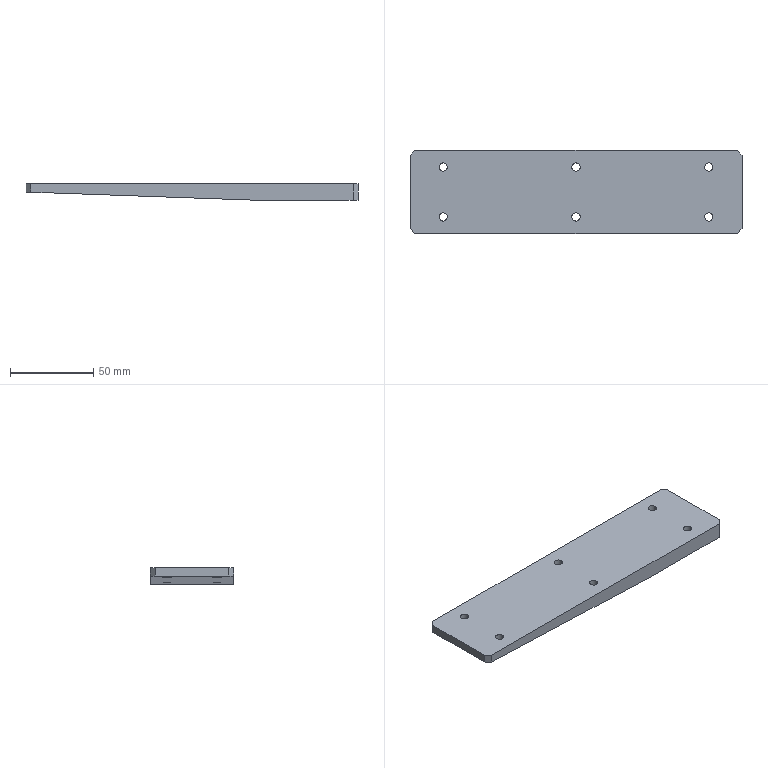Part | SolidWorks | features BaseBody 1 | 1 solid | 23 faces | box 200 x 50 x 10 mm | volume 81411 mm3 | cylinder 12 | plane 11 | commonest cylinder face diameters 5 x12
STEP:
#1=CARTESIAN_POINT('',(-82.5,15.,-0.625));
#2=VERTEX_POINT('',#1);
#3=CARTESIAN_POINT('',(-77.5,15.,-0.8036));
#4=VERTEX_POINT('',#3);
#5=CARTESIAN_POINT('',(-82.5,15.,-0.625));
#6=CARTESIAN_POINT('',(-82.5,10.,-0.625));
#7=CARTESIAN_POINT('',(-77.5,10.,-0.8036));
#8=CARTESIAN_POINT('',(-77.5,15.,-0.8036));
#9=(BOUNDED_CURVE()B_SPLINE_CURVE(3,(#5,#6,#7,#8),.UNSPECIFIED.,.F.,.F.)B_SPLINE_CURVE_WITH_KNOTS((4,4),(0.,3.142),.UNSPECIFIED.)CURVE()GEOMETRIC_REPRESENTATION_ITEM()RATIONAL_B_SPLINE_CURVE((1.,0.3333,0.3333,1.))REPRESENTATION_ITEM(''));
#10=EDGE_CURVE('',#2,#4,#9,.T.);
#11=ORIENTED_EDGE('',*,*,#10,.F.);
#12=CARTESIAN_POINT('',(-82.5,15.,5.));
#13=VERTEX_POINT('',#12);
#14=CARTESIAN_POINT('',(-82.5,15.,5.));
#15=DIRECTION('',(0.,0.,1.));
#16=VECTOR('',#15,1000.);
#17=LINE('',#14,#16);
#18=EDGE_CURVE('',#2,#13,#17,.T.);
#19=ORIENTED_EDGE('',*,*,#18,.T.);
#20=CARTESIAN_POINT('',(-77.5,15.,5.));
#21=VERTEX_POINT('',#20);
#22=CARTESIAN_POINT('',(-80.,15.,5.));
#23=DIRECTION('',(0.,0.,1.));
#24=DIRECTION('',(1.,0.,0.));
#25=AXIS2_PLACEMENT_3D('',#22,#23,#24);
#26=CIRCLE('',#25,2.5);
#27=EDGE_CURVE('',#13,#21,#26,.T.);
#28=ORIENTED_EDGE('',*,*,#27,.T.);
#29=CARTESIAN_POINT('',(-77.5,15.,5.));
#30=DIRECTION('',(0.,0.,1.));
#31=VECTOR('',#30,1000.);
#32=LINE('',#29,#31);
#33=EDGE_CURVE('',#4,#21,#32,.T.);
#34=ORIENTED_EDGE('',*,*,#33,.F.);
#35=EDGE_LOOP('',(#11,#19,#28,#34));
#36=FACE_OUTER_BOUND('',#35,.T.);
#37=CARTESIAN_POINT('',(-80.,15.,5.));
#38=DIRECTION('',(0.,0.,1.));
#39=DIRECTION('',(1.,0.,0.));
#40=AXIS2_PLACEMENT_3D('',#37,#38,#39);
#41=CYLINDRICAL_SURFACE('',#40,2.5);
#42=ADVANCED_FACE('',(#36),#41,.F.);
#43=CARTESIAN_POINT('',(-82.5,-15.,-0.625));
#44=VERTEX_POINT('',#43);
#45=CARTESIAN_POINT('',(-77.5,-15.,-0.8036));
#46=VERTEX_POINT('',#45);
#47=CARTESIAN_POINT('',(-82.5,-15.,-0.625));
#48=CARTESIAN_POINT('',(-82.5,-20.,-0.625));
#49=CARTESIAN_POINT('',(-77.5,-20.,-0.8036));
#50=CARTESIAN_POINT('',(-77.5,-15.,-0.8036));
#51=(BOUNDED_CURVE()B_SPLINE_CURVE(3,(#47,#48,#49,#50),.UNSPECIFIED.,.F.,.F.)B_SPLINE_CURVE_WITH_KNOTS((4,4),(0.,3.142),.UNSPECIFIED.)CURVE()GEOMETRIC_REPRESENTATION_ITEM()RATIONAL_B_SPLINE_CURVE((1.,0.3333,0.3333,1.))REPRESENTATION_ITEM(''));
#52=EDGE_CURVE('',#44,#46,#51,.T.);
#53=ORIENTED_EDGE('',*,*,#52,.F.);
#54=CARTESIAN_POINT('',(-82.5,-15.,5.));
#55=VERTEX_POINT('',#54);
#56=CARTESIAN_POINT('',(-82.5,-15.,5.));
#57=DIRECTION('',(0.,0.,1.));
#58=VECTOR('',#57,1000.);
#59=LINE('',#56,#58);
#60=EDGE_CURVE('',#44,#55,#59,.T.);
#61=ORIENTED_EDGE('',*,*,#60,.T.);
#62=CARTESIAN_POINT('',(-77.5,-15.,5.));
#63=VERTEX_POINT('',#62);
#64=CARTESIAN_POINT('',(-80.,-15.,5.));
#65=DIRECTION('',(0.,0.,1.));
#66=DIRECTION('',(1.,0.,0.));
#67=AXIS2_PLACEMENT_3D('',#64,#65,#66);
#68=CIRCLE('',#67,2.5);
#69=EDGE_CURVE('',#55,#63,#68,.T.);
#70=ORIENTED_EDGE('',*,*,#69,.T.);
#71=CARTESIAN_POINT('',(-77.5,-15.,5.));
#72=DIRECTION('',(0.,0.,1.));
#73=VECTOR('',#72,1000.);
#74=LINE('',#71,#73);
#75=EDGE_CURVE('',#46,#63,#74,.T.);
#76=ORIENTED_EDGE('',*,*,#75,.F.);
#77=EDGE_LOOP('',(#53,#61,#70,#76));
#78=FACE_OUTER_BOUND('',#77,.T.);
#79=CARTESIAN_POINT('',(-80.,-15.,5.));
#80=DIRECTION('',(0.,0.,1.));
#81=DIRECTION('',(1.,0.,0.));
#82=AXIS2_PLACEMENT_3D('',#79,#80,#81);
#83=CYLINDRICAL_SURFACE('',#82,2.5);
#84=ADVANCED_FACE('',(#78),#83,.F.);
#85=CARTESIAN_POINT('',(-2.5,15.,-3.482));
#86=VERTEX_POINT('',#85);
#87=CARTESIAN_POINT('',(2.5,15.,-3.661));
#88=VERTEX_POINT('',#87);
#89=CARTESIAN_POINT('',(-2.5,15.,-3.482));
#90=CARTESIAN_POINT('',(-2.5,10.,-3.482));
#91=CARTESIAN_POINT('',(2.5,10.,-3.661));
#92=CARTESIAN_POINT('',(2.5,15.,-3.661));
#93=(BOUNDED_CURVE()B_SPLINE_CURVE(3,(#89,#90,#91,#92),.UNSPECIFIED.,.F.,.T.)B_SPLINE_CURVE_WITH_KNOTS((4,4),(0.,3.142),.UNSPECIFIED.)CURVE()GEOMETRIC_REPRESENTATION_ITEM()RATIONAL_B_SPLINE_CURVE((1.,0.3333,0.3333,1.))REPRESENTATION_ITEM(''));
#94=EDGE_CURVE('',#86,#88,#93,.T.);
#95=ORIENTED_EDGE('',*,*,#94,.F.);
#96=CARTESIAN_POINT('',(-2.5,15.,5.));
#97=VERTEX_POINT('',#96);
#98=CARTESIAN_POINT('',(-2.5,15.,5.));
#99=DIRECTION('',(0.,0.,1.));
#100=VECTOR('',#99,1000.);
#101=LINE('',#98,#100);
#102=EDGE_CURVE('',#86,#97,#101,.T.);
#103=ORIENTED_EDGE('',*,*,#102,.T.);
#104=CARTESIAN_POINT('',(2.5,15.,5.));
#105=VERTEX_POINT('',#104);
#106=CARTESIAN_POINT('',(0.,15.,5.));
#107=DIRECTION('',(0.,0.,1.));
#108=DIRECTION('',(1.,0.,0.));
#109=AXIS2_PLACEMENT_3D('',#106,#107,#108);
#110=CIRCLE('',#109,2.5);
#111=EDGE_CURVE('',#97,#105,#110,.T.);
#112=ORIENTED_EDGE('',*,*,#111,.T.);
#113=CARTESIAN_POINT('',(2.5,15.,5.));
#114=DIRECTION('',(0.,0.,1.));
#115=VECTOR('',#114,1000.);
#116=LINE('',#113,#115);
#117=EDGE_CURVE('',#88,#105,#116,.T.);
#118=ORIENTED_EDGE('',*,*,#117,.F.);
#119=EDGE_LOOP('',(#95,#103,#112,#118));
#120=FACE_OUTER_BOUND('',#119,.T.);
#121=CARTESIAN_POINT('',(0.,15.,5.));
#122=DIRECTION('',(0.,0.,1.));
#123=DIRECTION('',(1.,0.,0.));
#124=AXIS2_PLACEMENT_3D('',#121,#122,#123);
#125=CYLINDRICAL_SURFACE('',#124,2.5);
#126=ADVANCED_FACE('',(#120),#125,.F.);
#127=CARTESIAN_POINT('',(-2.5,-15.,-3.482));
#128=VERTEX_POINT('',#127);
#129=CARTESIAN_POINT('',(2.5,-15.,-3.661));
#130=VERTEX_POINT('',#129);
#131=CARTESIAN_POINT('',(-2.5,-15.,-3.482));
#132=CARTESIAN_POINT('',(-2.5,-20.,-3.482));
#133=CARTESIAN_POINT('',(2.5,-20.,-3.661));
#134=CARTESIAN_POINT('',(2.5,-15.,-3.661));
#135=(BOUNDED_CURVE()B_SPLINE_CURVE(3,(#131,#132,#133,#134),.UNSPECIFIED.,.F.,.F.)B_SPLINE_CURVE_WITH_KNOTS((4,4),(0.,3.142),.UNSPECIFIED.)CURVE()GEOMETRIC_REPRESENTATION_ITEM()RATIONAL_B_SPLINE_CURVE((1.,0.3333,0.3333,1.))REPRESENTATION_ITEM(''));
#136=EDGE_CURVE('',#128,#130,#135,.T.);
#137=ORIENTED_EDGE('',*,*,#136,.F.);
#138=CARTESIAN_POINT('',(-2.5,-15.,5.));
#139=VERTEX_POINT('',#138);
#140=CARTESIAN_POINT('',(-2.5,-15.,5.));
#141=DIRECTION('',(0.,0.,1.));
#142=VECTOR('',#141,1000.);
#143=LINE('',#140,#142);
#144=EDGE_CURVE('',#128,#139,#143,.T.);
#145=ORIENTED_EDGE('',*,*,#144,.T.);
#146=CARTESIAN_POINT('',(2.5,-15.,5.));
#147=VERTEX_POINT('',#146);
#148=CARTESIAN_POINT('',(0.,-15.,5.));
#149=DIRECTION('',(0.,0.,1.));
#150=DIRECTION('',(1.,0.,0.));
#151=AXIS2_PLACEMENT_3D('',#148,#149,#150);
#152=CIRCLE('',#151,2.5);
#153=EDGE_CURVE('',#139,#147,#152,.T.);
#154=ORIENTED_EDGE('',*,*,#153,.T.);
#155=CARTESIAN_POINT('',(2.5,-15.,5.));
#156=DIRECTION('',(0.,0.,1.));
#157=VECTOR('',#156,1000.);
#158=LINE('',#155,#157);
#159=EDGE_CURVE('',#130,#147,#158,.T.);
#160=ORIENTED_EDGE('',*,*,#159,.F.);
#161=EDGE_LOOP('',(#137,#145,#154,#160));
#162=FACE_OUTER_BOUND('',#161,.T.);
#163=CARTESIAN_POINT('',(0.,-15.,5.));
#164=DIRECTION('',(0.,0.,1.));
#165=DIRECTION('',(1.,0.,0.));
#166=AXIS2_PLACEMENT_3D('',#163,#164,#165);
#167=CYLINDRICAL_SURFACE('',#166,2.5);
#168=ADVANCED_FACE('',(#162),#167,.F.);
#169=CARTESIAN_POINT('',(82.5,15.,-5.));
#170=VERTEX_POINT('',#169);
#171=CARTESIAN_POINT('',(77.5,15.,-5.));
#172=VERTEX_POINT('',#171);
#173=CARTESIAN_POINT('',(80.,15.,-5.));
#174=DIRECTION('',(0.,0.,-1.));
#175=DIRECTION('',(-1.,0.,0.));
#176=AXIS2_PLACEMENT_3D('',#173,#174,#175);
#177=CIRCLE('',#176,2.5);
#178=EDGE_CURVE('',#170,#172,#177,.T.);
#179=ORIENTED_EDGE('',*,*,#178,.T.);
#180=CARTESIAN_POINT('',(77.5,15.,5.));
#181=VERTEX_POINT('',#180);
#182=CARTESIAN_POINT('',(77.5,15.,5.));
#183=DIRECTION('',(0.,0.,1.));
#184=VECTOR('',#183,1000.);
#185=LINE('',#182,#184);
#186=EDGE_CURVE('',#172,#181,#185,.T.);
#187=ORIENTED_EDGE('',*,*,#186,.T.);
#188=CARTESIAN_POINT('',(82.5,15.,5.));
#189=VERTEX_POINT('',#188);
#190=CARTESIAN_POINT('',(80.,15.,5.));
#191=DIRECTION('',(0.,0.,1.));
#192=DIRECTION('',(1.,0.,0.));
#193=AXIS2_PLACEMENT_3D('',#190,#191,#192);
#194=CIRCLE('',#193,2.5);
#195=EDGE_CURVE('',#181,#189,#194,.T.);
#196=ORIENTED_EDGE('',*,*,#195,.T.);
#197=CARTESIAN_POINT('',(82.5,15.,5.));
#198=DIRECTION('',(0.,0.,1.));
#199=VECTOR('',#198,1000.);
#200=LINE('',#197,#199);
#201=EDGE_CURVE('',#170,#189,#200,.T.);
#202=ORIENTED_EDGE('',*,*,#201,.F.);
#203=EDGE_LOOP('',(#179,#187,#196,#202));
#204=FACE_OUTER_BOUND('',#203,.T.);
#205=CARTESIAN_POINT('',(80.,15.,5.));
#206=DIRECTION('',(0.,0.,1.));
#207=DIRECTION('',(1.,0.,0.));
#208=AXIS2_PLACEMENT_3D('',#205,#206,#207);
#209=CYLINDRICAL_SURFACE('',#208,2.5);
#210=ADVANCED_FACE('',(#204),#209,.F.);
#211=CARTESIAN_POINT('',(82.5,-15.,-5.));
#212=VERTEX_POINT('',#211);
#213=CARTESIAN_POINT('',(77.5,-15.,-5.));
#214=VERTEX_POINT('',#213);
#215=CARTESIAN_POINT('',(80.,-15.,-5.));
#216=DIRECTION('',(0.,0.,-1.));
#217=DIRECTION('',(-1.,0.,0.));
#218=AXIS2_PLACEMENT_3D('',#215,#216,#217);
#219=CIRCLE('',#218,2.5);
#220=EDGE_CURVE('',#212,#214,#219,.T.);
#221=ORIENTED_EDGE('',*,*,#220,.T.);
#222=CARTESIAN_POINT('',(77.5,-15.,5.));
#223=VERTEX_POINT('',#222);
#224=CARTESIAN_POINT('',(77.5,-15.,5.));
#225=DIRECTION('',(0.,0.,1.));
#226=VECTOR('',#225,1000.);
#227=LINE('',#224,#226);
#228=EDGE_CURVE('',#214,#223,#227,.T.);
#229=ORIENTED_EDGE('',*,*,#228,.T.);
#230=CARTESIAN_POINT('',(82.5,-15.,5.));
#231=VERTEX_POINT('',#230);
#232=CARTESIAN_POINT('',(80.,-15.,5.));
#233=DIRECTION('',(0.,0.,1.));
#234=DIRECTION('',(1.,0.,0.));
#235=AXIS2_PLACEMENT_3D('',#232,#233,#234);
#236=CIRCLE('',#235,2.5);
#237=EDGE_CURVE('',#223,#231,#236,.T.);
#238=ORIENTED_EDGE('',*,*,#237,.T.);
#239=CARTESIAN_POINT('',(82.5,-15.,5.));
#240=DIRECTION('',(0.,0.,1.));
#241=VECTOR('',#240,1000.);
#242=LINE('',#239,#241);
#243=EDGE_CURVE('',#212,#231,#242,.T.);
#244=ORIENTED_EDGE('',*,*,#243,.F.);
#245=EDGE_LOOP('',(#221,#229,#238,#244));
#246=FACE_OUTER_BOUND('',#245,.T.);
#247=CARTESIAN_POINT('',(80.,-15.,5.));
#248=DIRECTION('',(0.,0.,1.));
#249=DIRECTION('',(1.,0.,0.));
#250=AXIS2_PLACEMENT_3D('',#247,#248,#249);
#251=CYLINDRICAL_SURFACE('',#250,2.5);
#252=ADVANCED_FACE('',(#246),#251,.F.);
#253=CARTESIAN_POINT('',(-100.,-22.,0.));
#254=VERTEX_POINT('',#253);
#255=CARTESIAN_POINT('',(-100.,22.,0.));
#256=VERTEX_POINT('',#255);
#257=CARTESIAN_POINT('',(-100.,-25.,0.));
#258=DIRECTION('',(0.,1.,0.));
#259=VECTOR('',#258,1000.);
#260=LINE('',#257,#259);
#261=EDGE_CURVE('',#254,#256,#260,.T.);
#262=ORIENTED_EDGE('',*,*,#261,.F.);
#263=CARTESIAN_POINT('',(-100.,-22.,5.));
#264=VERTEX_POINT('',#263);
#265=CARTESIAN_POINT('',(-100.,-22.,5.));
#266=DIRECTION('',(0.,0.,1.));
#267=VECTOR('',#266,1000.);
#268=LINE('',#265,#267);
#269=EDGE_CURVE('',#254,#264,#268,.T.);
#270=ORIENTED_EDGE('',*,*,#269,.T.);
#271=CARTESIAN_POINT('',(-100.,22.,5.));
#272=VERTEX_POINT('',#271);
#273=CARTESIAN_POINT('',(-100.,25.,5.));
#274=DIRECTION('',(0.,-1.,0.));
#275=VECTOR('',#274,1000.);
#276=LINE('',#273,#275);
#277=EDGE_CURVE('',#272,#264,#276,.T.);
#278=ORIENTED_EDGE('',*,*,#277,.F.);
#279=CARTESIAN_POINT('',(-100.,22.,5.));
#280=DIRECTION('',(0.,0.,-1.));
#281=VECTOR('',#280,1000.);
#282=LINE('',#279,#281);
#283=EDGE_CURVE('',#272,#256,#282,.T.);
#284=ORIENTED_EDGE('',*,*,#283,.T.);
#285=EDGE_LOOP('',(#262,#270,#278,#284));
#286=FACE_OUTER_BOUND('',#285,.T.);
#287=CARTESIAN_POINT('',(-100.,25.,5.));
#288=DIRECTION('',(1.,0.,0.));
#289=DIRECTION('',(0.,0.,-1.));
#290=AXIS2_PLACEMENT_3D('',#287,#288,#289);
#291=PLANE('',#290);
#292=ADVANCED_FACE('',(#286),#291,.F.);
#293=CARTESIAN_POINT('',(40.,-25.,-5.));
#294=VERTEX_POINT('',#293);
#295=CARTESIAN_POINT('',(97.,-25.,-5.));
#296=VERTEX_POINT('',#295);
#297=CARTESIAN_POINT('',(100.,-25.,-5.));
#298=DIRECTION('',(1.,0.,0.));
#299=VECTOR('',#298,1000.);
#300=LINE('',#297,#299);
#301=EDGE_CURVE('',#294,#296,#300,.T.);
#302=ORIENTED_EDGE('',*,*,#301,.T.);
#303=CARTESIAN_POINT('',(97.,-25.,5.));
#304=VERTEX_POINT('',#303);
#305=CARTESIAN_POINT('',(97.,-25.,5.));
#306=DIRECTION('',(0.,0.,1.));
#307=VECTOR('',#306,1000.);
#308=LINE('',#305,#307);
#309=EDGE_CURVE('',#296,#304,#308,.T.);
#310=ORIENTED_EDGE('',*,*,#309,.T.);
#311=CARTESIAN_POINT('',(-97.,-25.,5.));
#312=VERTEX_POINT('',#311);
#313=CARTESIAN_POINT('',(100.,-25.,5.));
#314=DIRECTION('',(1.,0.,0.));
#315=VECTOR('',#314,1000.);
#316=LINE('',#313,#315);
#317=EDGE_CURVE('',#312,#304,#316,.T.);
#318=ORIENTED_EDGE('',*,*,#317,.F.);
#319=CARTESIAN_POINT('',(-97.,-25.,-0.1071));
#320=VERTEX_POINT('',#319);
#321=CARTESIAN_POINT('',(-97.,-25.,5.));
#322=DIRECTION('',(0.,0.,-1.));
#323=VECTOR('',#322,1000.);
#324=LINE('',#321,#323);
#325=EDGE_CURVE('',#312,#320,#324,.T.);
#326=ORIENTED_EDGE('',*,*,#325,.T.);
#327=CARTESIAN_POINT('',(-100.,-25.,0.));
#328=DIRECTION('',(0.9994,0.,-0.03569));
#329=VECTOR('',#328,1000.);
#330=LINE('',#327,#329);
#331=EDGE_CURVE('',#320,#294,#330,.T.);
#332=ORIENTED_EDGE('',*,*,#331,.T.);
#333=EDGE_LOOP('',(#302,#310,#318,#326,#332));
#334=FACE_OUTER_BOUND('',#333,.T.);
#335=CARTESIAN_POINT('',(100.,-25.,5.));
#336=DIRECTION('',(0.,1.,0.));
#337=DIRECTION('',(-1.,0.,0.));
#338=AXIS2_PLACEMENT_3D('',#335,#336,#337);
#339=PLANE('',#338);
#340=ADVANCED_FACE('',(#334),#339,.F.);
#341=CARTESIAN_POINT('',(100.,-22.,5.));
#342=VERTEX_POINT('',#341);
#343=CARTESIAN_POINT('',(100.,22.,5.));
#344=VERTEX_POINT('',#343);
#345=CARTESIAN_POINT('',(100.,25.,5.));
#346=DIRECTION('',(0.,1.,0.));
#347=VECTOR('',#346,1000.);
#348=LINE('',#345,#347);
#349=EDGE_CURVE('',#342,#344,#348,.T.);
#350=ORIENTED_EDGE('',*,*,#349,.F.);
#351=CARTESIAN_POINT('',(100.,-22.,-5.));
#352=VERTEX_POINT('',#351);
#353=CARTESIAN_POINT('',(100.,-22.,5.));
#354=DIRECTION('',(0.,0.,-1.));
#355=VECTOR('',#354,1000.);
#356=LINE('',#353,#355);
#357=EDGE_CURVE('',#342,#352,#356,.T.);
#358=ORIENTED_EDGE('',*,*,#357,.T.);
#359=CARTESIAN_POINT('',(100.,22.,-5.));
#360=VERTEX_POINT('',#359);
#361=CARTESIAN_POINT('',(100.,25.,-5.));
#362=DIRECTION('',(0.,1.,0.));
#363=VECTOR('',#362,1000.);
#364=LINE('',#361,#363);
#365=EDGE_CURVE('',#352,#360,#364,.T.);
#366=ORIENTED_EDGE('',*,*,#365,.T.);
#367=CARTESIAN_POINT('',(100.,22.,5.));
#368=DIRECTION('',(0.,0.,1.));
#369=VECTOR('',#368,1000.);
#370=LINE('',#367,#369);
#371=EDGE_CURVE('',#360,#344,#370,.T.);
#372=ORIENTED_EDGE('',*,*,#371,.T.);
#373=EDGE_LOOP('',(#350,#358,#366,#372));
#374=FACE_OUTER_BOUND('',#373,.T.);
#375=CARTESIAN_POINT('',(100.,25.,5.));
#376=DIRECTION('',(-1.,0.,0.));
#377=DIRECTION('',(0.,0.,1.));
#378=AXIS2_PLACEMENT_3D('',#375,#376,#377);
#379=PLANE('',#378);
#380=ADVANCED_FACE('',(#374),#379,.F.);
#381=CARTESIAN_POINT('',(97.,25.,5.));
#382=VERTEX_POINT('',#381);
#383=CARTESIAN_POINT('',(-97.,25.,5.));
#384=VERTEX_POINT('',#383);
#385=CARTESIAN_POINT('',(100.,25.,5.));
#386=DIRECTION('',(-1.,0.,0.));
#387=VECTOR('',#386,1000.);
#388=LINE('',#385,#387);
#389=EDGE_CURVE('',#382,#384,#388,.T.);
#390=ORIENTED_EDGE('',*,*,#389,.F.);
#391=CARTESIAN_POINT('',(97.,25.,-5.));
#392=VERTEX_POINT('',#391);
#393=CARTESIAN_POINT('',(97.,25.,5.));
#394=DIRECTION('',(0.,0.,-1.));
#395=VECTOR('',#394,1000.);
#396=LINE('',#393,#395);
#397=EDGE_CURVE('',#382,#392,#396,.T.);
#398=ORIENTED_EDGE('',*,*,#397,.T.);
#399=CARTESIAN_POINT('',(40.,25.,-5.));
#400=VERTEX_POINT('',#399);
#401=CARTESIAN_POINT('',(100.,25.,-5.));
#402=DIRECTION('',(-1.,0.,0.));
#403=VECTOR('',#402,1000.);
#404=LINE('',#401,#403);
#405=EDGE_CURVE('',#392,#400,#404,.T.);
#406=ORIENTED_EDGE('',*,*,#405,.T.);
#407=CARTESIAN_POINT('',(-97.,25.,-0.1071));
#408=VERTEX_POINT('',#407);
#409=CARTESIAN_POINT('',(-100.,25.,0.));
#410=DIRECTION('',(0.9994,0.,-0.03569));
#411=VECTOR('',#410,1000.);
#412=LINE('',#409,#411);
#413=EDGE_CURVE('',#408,#400,#412,.T.);
#414=ORIENTED_EDGE('',*,*,#413,.F.);
#415=CARTESIAN_POINT('',(-97.,25.,5.));
#416=DIRECTION('',(0.,0.,1.));
#417=VECTOR('',#416,1000.);
#418=LINE('',#415,#417);
#419=EDGE_CURVE('',#408,#384,#418,.T.);
#420=ORIENTED_EDGE('',*,*,#419,.T.);
#421=EDGE_LOOP('',(#390,#398,#406,#414,#420));
#422=FACE_OUTER_BOUND('',#421,.T.);
#423=CARTESIAN_POINT('',(100.,25.,5.));
#424=DIRECTION('',(0.,-1.,0.));
#425=DIRECTION('',(1.,0.,0.));
#426=AXIS2_PLACEMENT_3D('',#423,#424,#425);
#427=PLANE('',#426);
#428=ADVANCED_FACE('',(#422),#427,.F.);
#429=CARTESIAN_POINT('',(-80.,15.,5.));
#430=DIRECTION('',(0.,0.,1.));
#431=DIRECTION('',(1.,0.,0.));
#432=AXIS2_PLACEMENT_3D('',#429,#430,#431);
#433=CIRCLE('',#432,2.5);
#434=EDGE_CURVE('',#21,#13,#433,.T.);
#435=ORIENTED_EDGE('',*,*,#434,.F.);
#436=ORIENTED_EDGE('',*,*,#27,.F.);
#437=EDGE_LOOP('',(#435,#436));
#438=FACE_BOUND('',#437,.T.);
#439=CARTESIAN_POINT('',(-80.,-15.,5.));
#440=DIRECTION('',(0.,0.,1.));
#441=DIRECTION('',(1.,0.,0.));
#442=AXIS2_PLACEMENT_3D('',#439,#440,#441);
#443=CIRCLE('',#442,2.5);
#444=EDGE_CURVE('',#63,#55,#443,.T.);
#445=ORIENTED_EDGE('',*,*,#444,.F.);
#446=ORIENTED_EDGE('',*,*,#69,.F.);
#447=EDGE_LOOP('',(#445,#446));
#448=FACE_BOUND('',#447,.T.);
#449=CARTESIAN_POINT('',(0.,15.,5.));
#450=DIRECTION('',(0.,0.,1.));
#451=DIRECTION('',(1.,0.,0.));
#452=AXIS2_PLACEMENT_3D('',#449,#450,#451);
#453=CIRCLE('',#452,2.5);
#454=EDGE_CURVE('',#105,#97,#453,.T.);
#455=ORIENTED_EDGE('',*,*,#454,.F.);
#456=ORIENTED_EDGE('',*,*,#111,.F.);
#457=EDGE_LOOP('',(#455,#456));
#458=FACE_BOUND('',#457,.T.);
#459=CARTESIAN_POINT('',(0.,-15.,5.));
#460=DIRECTION('',(0.,0.,1.));
#461=DIRECTION('',(1.,0.,0.));
#462=AXIS2_PLACEMENT_3D('',#459,#460,#461);
#463=CIRCLE('',#462,2.5);
#464=EDGE_CURVE('',#147,#139,#463,.T.);
#465=ORIENTED_EDGE('',*,*,#464,.F.);
#466=ORIENTED_EDGE('',*,*,#153,.F.);
#467=EDGE_LOOP('',(#465,#466));
#468=FACE_BOUND('',#467,.T.);
#469=CARTESIAN_POINT('',(80.,15.,5.));
#470=DIRECTION('',(0.,0.,1.));
#471=DIRECTION('',(1.,0.,0.));
#472=AXIS2_PLACEMENT_3D('',#469,#470,#471);
#473=CIRCLE('',#472,2.5);
#474=EDGE_CURVE('',#189,#181,#473,.T.);
#475=ORIENTED_EDGE('',*,*,#474,.F.);
#476=ORIENTED_EDGE('',*,*,#195,.F.);
#477=EDGE_LOOP('',(#475,#476));
#478=FACE_BOUND('',#477,.T.);
#479=CARTESIAN_POINT('',(80.,-15.,5.));
#480=DIRECTION('',(0.,0.,1.));
#481=DIRECTION('',(1.,0.,0.));
#482=AXIS2_PLACEMENT_3D('',#479,#480,#481);
#483=CIRCLE('',#482,2.5);
#484=EDGE_CURVE('',#231,#223,#483,.T.);
#485=ORIENTED_EDGE('',*,*,#484,.F.);
#486=ORIENTED_EDGE('',*,*,#237,.F.);
#487=EDGE_LOOP('',(#485,#486));
#488=FACE_BOUND('',#487,.T.);
#489=ORIENTED_EDGE('',*,*,#317,.T.);
#490=CARTESIAN_POINT('',(100.,-22.,5.));
#491=DIRECTION('',(0.7071,0.7071,0.));
#492=VECTOR('',#491,1000.);
#493=LINE('',#490,#492);
#494=EDGE_CURVE('',#304,#342,#493,.T.);
#495=ORIENTED_EDGE('',*,*,#494,.T.);
#496=ORIENTED_EDGE('',*,*,#349,.T.);
#497=CARTESIAN_POINT('',(97.,25.,5.));
#498=DIRECTION('',(-0.7071,0.7071,0.));
#499=VECTOR('',#498,1000.);
#500=LINE('',#497,#499);
#501=EDGE_CURVE('',#344,#382,#500,.T.);
#502=ORIENTED_EDGE('',*,*,#501,.T.);
#503=ORIENTED_EDGE('',*,*,#389,.T.);
#504=CARTESIAN_POINT('',(-100.,22.,5.));
#505=DIRECTION('',(-0.7071,-0.7071,0.));
#506=VECTOR('',#505,1000.);
#507=LINE('',#504,#506);
#508=EDGE_CURVE('',#384,#272,#507,.T.);
#509=ORIENTED_EDGE('',*,*,#508,.T.);
#510=ORIENTED_EDGE('',*,*,#277,.T.);
#511=CARTESIAN_POINT('',(-97.,-25.,5.));
#512=DIRECTION('',(0.7071,-0.7071,0.));
#513=VECTOR('',#512,1000.);
#514=LINE('',#511,#513);
#515=EDGE_CURVE('',#264,#312,#514,.T.);
#516=ORIENTED_EDGE('',*,*,#515,.T.);
#517=EDGE_LOOP('',(#489,#495,#496,#502,#503,#509,#510,#516));
#518=FACE_OUTER_BOUND('',#517,.T.);
#519=CARTESIAN_POINT('',(-100.,-25.,5.));
#520=DIRECTION('',(0.,0.,-1.));
#521=DIRECTION('',(-1.,0.,0.));
#522=AXIS2_PLACEMENT_3D('',#519,#520,#521);
#523=PLANE('',#522);
#524=ADVANCED_FACE('',(#438,#448,#458,#468,#478,#488,#518),#523,.F.);
#525=ORIENTED_EDGE('',*,*,#178,.F.);
#526=CARTESIAN_POINT('',(80.,15.,-5.));
#527=DIRECTION('',(0.,0.,-1.));
#528=DIRECTION('',(-1.,0.,0.));
#529=AXIS2_PLACEMENT_3D('',#526,#527,#528);
#530=CIRCLE('',#529,2.5);
#531=EDGE_CURVE('',#172,#170,#530,.T.);
#532=ORIENTED_EDGE('',*,*,#531,.F.);
#533=EDGE_LOOP('',(#525,#532));
#534=FACE_BOUND('',#533,.T.);
#535=ORIENTED_EDGE('',*,*,#220,.F.);
#536=CARTESIAN_POINT('',(80.,-15.,-5.));
#537=DIRECTION('',(0.,0.,-1.));
#538=DIRECTION('',(-1.,0.,0.));
#539=AXIS2_PLACEMENT_3D('',#536,#537,#538);
#540=CIRCLE('',#539,2.5);
#541=EDGE_CURVE('',#214,#212,#540,.T.);
#542=ORIENTED_EDGE('',*,*,#541,.F.);
#543=EDGE_LOOP('',(#535,#542));
#544=FACE_BOUND('',#543,.T.);
#545=ORIENTED_EDGE('',*,*,#365,.F.);
#546=CARTESIAN_POINT('',(-1.5,-123.5,-5.));
#547=DIRECTION('',(-0.7071,-0.7071,0.));
#548=VECTOR('',#547,1000.);
#549=LINE('',#546,#548);
#550=EDGE_CURVE('',#352,#296,#549,.T.);
#551=ORIENTED_EDGE('',*,*,#550,.T.);
#552=ORIENTED_EDGE('',*,*,#301,.F.);
#553=CARTESIAN_POINT('',(40.,-25.,-5.));
#554=DIRECTION('',(0.,1.,0.));
#555=VECTOR('',#554,1000.);
#556=LINE('',#553,#555);
#557=EDGE_CURVE('',#294,#400,#556,.T.);
#558=ORIENTED_EDGE('',*,*,#557,.T.);
#559=ORIENTED_EDGE('',*,*,#405,.F.);
#560=CARTESIAN_POINT('',(23.5,98.5,-5.));
#561=DIRECTION('',(0.7071,-0.7071,0.));
#562=VECTOR('',#561,1000.);
#563=LINE('',#560,#562);
#564=EDGE_CURVE('',#392,#360,#563,.T.);
#565=ORIENTED_EDGE('',*,*,#564,.T.);
#566=EDGE_LOOP('',(#545,#551,#552,#558,#559,#565));
#567=FACE_OUTER_BOUND('',#566,.T.);
#568=CARTESIAN_POINT('',(-100.,-25.,-5.));
#569=DIRECTION('',(0.,0.,-1.));
#570=DIRECTION('',(-1.,0.,0.));
#571=AXIS2_PLACEMENT_3D('',#568,#569,#570);
#572=PLANE('',#571);
#573=ADVANCED_FACE('',(#534,#544,#567),#572,.T.);
#574=CARTESIAN_POINT('',(-77.5,15.,-0.8036));
#575=CARTESIAN_POINT('',(-77.5,20.,-0.8036));
#576=CARTESIAN_POINT('',(-82.5,20.,-0.625));
#577=CARTESIAN_POINT('',(-82.5,15.,-0.625));
#578=(BOUNDED_CURVE()B_SPLINE_CURVE(3,(#574,#575,#576,#577),.UNSPECIFIED.,.F.,.F.)B_SPLINE_CURVE_WITH_KNOTS((4,4),(3.142,6.283),.UNSPECIFIED.)CURVE()GEOMETRIC_REPRESENTATION_ITEM()RATIONAL_B_SPLINE_CURVE((1.,0.3333,0.3333,1.))REPRESENTATION_ITEM(''));
#579=EDGE_CURVE('',#4,#2,#578,.T.);
#580=ORIENTED_EDGE('',*,*,#579,.T.);
#581=ORIENTED_EDGE('',*,*,#10,.T.);
#582=EDGE_LOOP('',(#580,#581));
#583=FACE_BOUND('',#582,.T.);
#584=CARTESIAN_POINT('',(-77.5,-15.,-0.8036));
#585=CARTESIAN_POINT('',(-77.5,-10.,-0.8036));
#586=CARTESIAN_POINT('',(-82.5,-10.,-0.625));
#587=CARTESIAN_POINT('',(-82.5,-15.,-0.625));
#588=(BOUNDED_CURVE()B_SPLINE_CURVE(3,(#584,#585,#586,#587),.UNSPECIFIED.,.F.,.F.)B_SPLINE_CURVE_WITH_KNOTS((4,4),(3.142,6.283),.UNSPECIFIED.)CURVE()GEOMETRIC_REPRESENTATION_ITEM()RATIONAL_B_SPLINE_CURVE((1.,0.3333,0.3333,1.))REPRESENTATION_ITEM(''));
#589=EDGE_CURVE('',#46,#44,#588,.T.);
#590=ORIENTED_EDGE('',*,*,#589,.T.);
#591=ORIENTED_EDGE('',*,*,#52,.T.);
#592=EDGE_LOOP('',(#590,#591));
#593=FACE_BOUND('',#592,.T.);
#594=CARTESIAN_POINT('',(2.5,15.,-3.661));
#595=CARTESIAN_POINT('',(2.5,20.,-3.661));
#596=CARTESIAN_POINT('',(-2.5,20.,-3.482));
#597=CARTESIAN_POINT('',(-2.5,15.,-3.482));
#598=(BOUNDED_CURVE()B_SPLINE_CURVE(3,(#594,#595,#596,#597),.UNSPECIFIED.,.F.,.F.)B_SPLINE_CURVE_WITH_KNOTS((4,4),(3.142,6.283),.UNSPECIFIED.)CURVE()GEOMETRIC_REPRESENTATION_ITEM()RATIONAL_B_SPLINE_CURVE((1.,0.3333,0.3333,1.))REPRESENTATION_ITEM(''));
#599=EDGE_CURVE('',#88,#86,#598,.T.);
#600=ORIENTED_EDGE('',*,*,#599,.T.);
#601=ORIENTED_EDGE('',*,*,#94,.T.);
#602=EDGE_LOOP('',(#600,#601));
#603=FACE_BOUND('',#602,.T.);
#604=CARTESIAN_POINT('',(2.5,-15.,-3.661));
#605=CARTESIAN_POINT('',(2.5,-10.,-3.661));
#606=CARTESIAN_POINT('',(-2.5,-10.,-3.482));
#607=CARTESIAN_POINT('',(-2.5,-15.,-3.482));
#608=(BOUNDED_CURVE()B_SPLINE_CURVE(3,(#604,#605,#606,#607),.UNSPECIFIED.,.F.,.F.)B_SPLINE_CURVE_WITH_KNOTS((4,4),(3.142,6.283),.UNSPECIFIED.)CURVE()GEOMETRIC_REPRESENTATION_ITEM()RATIONAL_B_SPLINE_CURVE((1.,0.3333,0.3333,1.))REPRESENTATION_ITEM(''));
#609=EDGE_CURVE('',#130,#128,#608,.T.);
#610=ORIENTED_EDGE('',*,*,#609,.T.);
#611=ORIENTED_EDGE('',*,*,#136,.T.);
#612=EDGE_LOOP('',(#610,#611));
#613=FACE_BOUND('',#612,.T.);
#614=ORIENTED_EDGE('',*,*,#331,.F.);
#615=CARTESIAN_POINT('',(-97.091,-24.909,-0.1039));
#616=DIRECTION('',(-0.7069,0.7069,0.02525));
#617=VECTOR('',#616,1000.);
#618=LINE('',#615,#617);
#619=EDGE_CURVE('',#320,#254,#618,.T.);
#620=ORIENTED_EDGE('',*,*,#619,.T.);
#621=ORIENTED_EDGE('',*,*,#261,.T.);
#622=CARTESIAN_POINT('',(-100.089,21.911,0.003187));
#623=DIRECTION('',(0.7069,0.7069,-0.02525));
#624=VECTOR('',#623,1000.);
#625=LINE('',#622,#624);
#626=EDGE_CURVE('',#256,#408,#625,.T.);
#627=ORIENTED_EDGE('',*,*,#626,.T.);
#628=ORIENTED_EDGE('',*,*,#413,.T.);
#629=ORIENTED_EDGE('',*,*,#557,.F.);
#630=EDGE_LOOP('',(#614,#620,#621,#627,#628,#629));
#631=FACE_OUTER_BOUND('',#630,.T.);
#632=CARTESIAN_POINT('',(-100.,-25.,0.));
#633=DIRECTION('',(0.03569,0.,0.9994));
#634=DIRECTION('',(0.9994,0.,-0.03569));
#635=AXIS2_PLACEMENT_3D('',#632,#633,#634);
#636=PLANE('',#635);
#637=ADVANCED_FACE('',(#583,#593,#603,#613,#631),#636,.F.);
#638=ORIENTED_EDGE('',*,*,#494,.F.);
#639=ORIENTED_EDGE('',*,*,#309,.F.);
#640=ORIENTED_EDGE('',*,*,#550,.F.);
#641=ORIENTED_EDGE('',*,*,#357,.F.);
#642=EDGE_LOOP('',(#638,#639,#640,#641));
#643=FACE_OUTER_BOUND('',#642,.T.);
#644=CARTESIAN_POINT('',(100.,-22.,5.));
#645=DIRECTION('',(-0.7071,0.7071,0.));
#646=DIRECTION('',(-0.7071,-0.7071,0.));
#647=AXIS2_PLACEMENT_3D('',#644,#645,#646);
#648=PLANE('',#647);
#649=ADVANCED_FACE('',(#643),#648,.F.);
#650=ORIENTED_EDGE('',*,*,#501,.F.);
#651=ORIENTED_EDGE('',*,*,#371,.F.);
#652=ORIENTED_EDGE('',*,*,#564,.F.);
#653=ORIENTED_EDGE('',*,*,#397,.F.);
#654=EDGE_LOOP('',(#650,#651,#652,#653));
#655=FACE_OUTER_BOUND('',#654,.T.);
#656=CARTESIAN_POINT('',(97.,25.,5.));
#657=DIRECTION('',(-0.7071,-0.7071,0.));
#658=DIRECTION('',(0.7071,-0.7071,0.));
#659=AXIS2_PLACEMENT_3D('',#656,#657,#658);
#660=PLANE('',#659);
#661=ADVANCED_FACE('',(#655),#660,.F.);
#662=ORIENTED_EDGE('',*,*,#515,.F.);
#663=ORIENTED_EDGE('',*,*,#269,.F.);
#664=ORIENTED_EDGE('',*,*,#619,.F.);
#665=ORIENTED_EDGE('',*,*,#325,.F.);
#666=EDGE_LOOP('',(#662,#663,#664,#665));
#667=FACE_OUTER_BOUND('',#666,.T.);
#668=CARTESIAN_POINT('',(-97.,-25.,5.));
#669=DIRECTION('',(0.7071,0.7071,0.));
#670=DIRECTION('',(-0.7071,0.7071,0.));
#671=AXIS2_PLACEMENT_3D('',#668,#669,#670);
#672=PLANE('',#671);
#673=ADVANCED_FACE('',(#667),#672,.F.);
#674=ORIENTED_EDGE('',*,*,#508,.F.);
#675=ORIENTED_EDGE('',*,*,#419,.F.);
#676=ORIENTED_EDGE('',*,*,#626,.F.);
#677=ORIENTED_EDGE('',*,*,#283,.F.);
#678=EDGE_LOOP('',(#674,#675,#676,#677));
#679=FACE_OUTER_BOUND('',#678,.T.);
#680=CARTESIAN_POINT('',(-100.,22.,5.));
#681=DIRECTION('',(0.7071,-0.7071,0.));
#682=DIRECTION('',(0.7071,0.7071,0.));
#683=AXIS2_PLACEMENT_3D('',#680,#681,#682);
#684=PLANE('',#683);
#685=ADVANCED_FACE('',(#679),#684,.F.);
#686=ORIENTED_EDGE('',*,*,#228,.F.);
#687=ORIENTED_EDGE('',*,*,#541,.T.);
#688=ORIENTED_EDGE('',*,*,#243,.T.);
#689=ORIENTED_EDGE('',*,*,#484,.T.);
#690=EDGE_LOOP('',(#686,#687,#688,#689));
#691=FACE_OUTER_BOUND('',#690,.T.);
#692=CARTESIAN_POINT('',(80.,-15.,5.));
#693=DIRECTION('',(0.,0.,1.));
#694=DIRECTION('',(1.,0.,0.));
#695=AXIS2_PLACEMENT_3D('',#692,#693,#694);
#696=CYLINDRICAL_SURFACE('',#695,2.5);
#697=ADVANCED_FACE('',(#691),#696,.F.);
#698=ORIENTED_EDGE('',*,*,#186,.F.);
#699=ORIENTED_EDGE('',*,*,#531,.T.);
#700=ORIENTED_EDGE('',*,*,#201,.T.);
#701=ORIENTED_EDGE('',*,*,#474,.T.);
#702=EDGE_LOOP('',(#698,#699,#700,#701));
#703=FACE_OUTER_BOUND('',#702,.T.);
#704=CARTESIAN_POINT('',(80.,15.,5.));
#705=DIRECTION('',(0.,0.,1.));
#706=DIRECTION('',(1.,0.,0.));
#707=AXIS2_PLACEMENT_3D('',#704,#705,#706);
#708=CYLINDRICAL_SURFACE('',#707,2.5);
#709=ADVANCED_FACE('',(#703),#708,.F.);
#710=ORIENTED_EDGE('',*,*,#144,.F.);
#711=ORIENTED_EDGE('',*,*,#609,.F.);
#712=ORIENTED_EDGE('',*,*,#159,.T.);
#713=ORIENTED_EDGE('',*,*,#464,.T.);
#714=EDGE_LOOP('',(#710,#711,#712,#713));
#715=FACE_OUTER_BOUND('',#714,.T.);
#716=CARTESIAN_POINT('',(0.,-15.,5.));
#717=DIRECTION('',(0.,0.,1.));
#718=DIRECTION('',(1.,0.,0.));
#719=AXIS2_PLACEMENT_3D('',#716,#717,#718);
#720=CYLINDRICAL_SURFACE('',#719,2.5);
#721=ADVANCED_FACE('',(#715),#720,.F.);
#722=ORIENTED_EDGE('',*,*,#102,.F.);
#723=ORIENTED_EDGE('',*,*,#599,.F.);
#724=ORIENTED_EDGE('',*,*,#117,.T.);
#725=ORIENTED_EDGE('',*,*,#454,.T.);
#726=EDGE_LOOP('',(#722,#723,#724,#725));
#727=FACE_OUTER_BOUND('',#726,.T.);
#728=CARTESIAN_POINT('',(0.,15.,5.));
#729=DIRECTION('',(0.,0.,1.));
#730=DIRECTION('',(1.,0.,0.));
#731=AXIS2_PLACEMENT_3D('',#728,#729,#730);
#732=CYLINDRICAL_SURFACE('',#731,2.5);
#733=ADVANCED_FACE('',(#727),#732,.F.);
#734=ORIENTED_EDGE('',*,*,#60,.F.);
#735=ORIENTED_EDGE('',*,*,#589,.F.);
#736=ORIENTED_EDGE('',*,*,#75,.T.);
#737=ORIENTED_EDGE('',*,*,#444,.T.);
#738=EDGE_LOOP('',(#734,#735,#736,#737));
#739=FACE_OUTER_BOUND('',#738,.T.);
#740=CARTESIAN_POINT('',(-80.,-15.,5.));
#741=DIRECTION('',(0.,0.,1.));
#742=DIRECTION('',(1.,0.,0.));
#743=AXIS2_PLACEMENT_3D('',#740,#741,#742);
#744=CYLINDRICAL_SURFACE('',#743,2.5);
#745=ADVANCED_FACE('',(#739),#744,.F.);
#746=ORIENTED_EDGE('',*,*,#18,.F.);
#747=ORIENTED_EDGE('',*,*,#579,.F.);
#748=ORIENTED_EDGE('',*,*,#33,.T.);
#749=ORIENTED_EDGE('',*,*,#434,.T.);
#750=EDGE_LOOP('',(#746,#747,#748,#749));
#751=FACE_OUTER_BOUND('',#750,.T.);
#752=CARTESIAN_POINT('',(-80.,15.,5.));
#753=DIRECTION('',(0.,0.,1.));
#754=DIRECTION('',(1.,0.,0.));
#755=AXIS2_PLACEMENT_3D('',#752,#753,#754);
#756=CYLINDRICAL_SURFACE('',#755,2.5);
#757=ADVANCED_FACE('',(#751),#756,.F.);
#758=CLOSED_SHELL('',(#42,#84,#126,#168,#210,#252,#292,#340,#380,#428,#524,#573,#637,#649,#661,#673,#685,#697,#709,#721,#733,#745,#757));
#759=MANIFOLD_SOLID_BREP('',#758);
#760=CARTESIAN_POINT('',(0.,0.,0.));
#761=DIRECTION('',(0.,0.,1.));
#762=DIRECTION('',(1.,0.,0.));
#763=AXIS2_PLACEMENT_3D('',#760,#761,#762);
#764=(LENGTH_UNIT()NAMED_UNIT(*)SI_UNIT(.MILLI.,.METRE.));
#765=UNCERTAINTY_MEASURE_WITH_UNIT(LENGTH_MEASURE(0.00001),#764,'','');
#766=(NAMED_UNIT(*)PLANE_ANGLE_UNIT()SI_UNIT($,.RADIAN.));
#767=(NAMED_UNIT(*)SI_UNIT($,.STERADIAN.)SOLID_ANGLE_UNIT());
#768=(GEOMETRIC_REPRESENTATION_CONTEXT(3)GLOBAL_UNCERTAINTY_ASSIGNED_CONTEXT((#765))GLOBAL_UNIT_ASSIGNED_CONTEXT((#764,#766,#767))REPRESENTATION_CONTEXT('',''));
#769=ADVANCED_BREP_SHAPE_REPRESENTATION('',(#759,#763),#768);